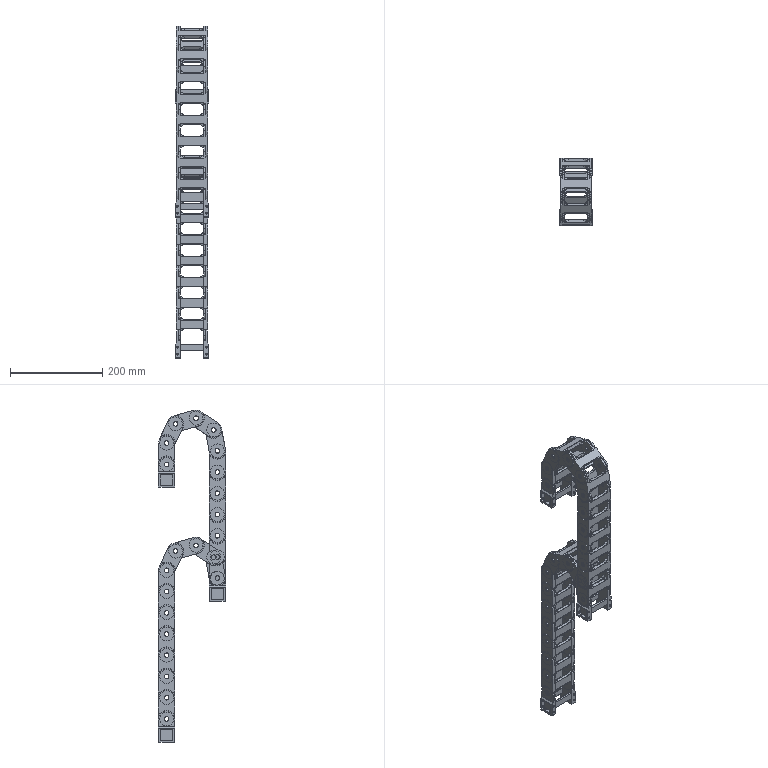Part | SolidWorks | features BaseBody 13, LPattern 3 | 25 solids | 5762 faces | volume 907035 mm3 | cylinder 3130 | plane 2632 | commonest cylinder face diameters 2 x943 4.24 x264 18.2 x188 32.34 x182 10 x176 13.7 x176